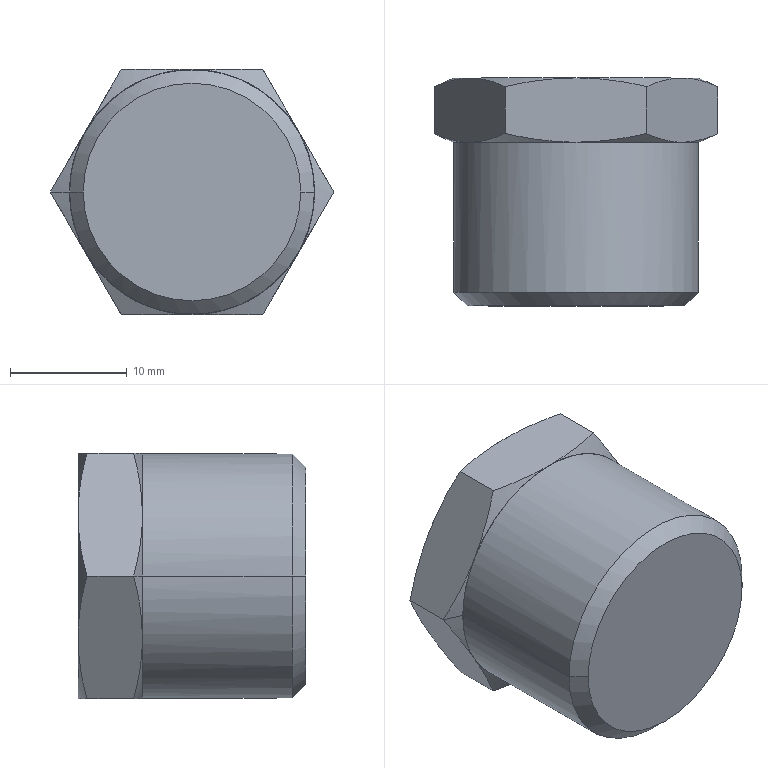Part | SolidWorks | features BaseBody 1 | 1 solid | 27 faces | box 24.249 x 19.5 x 21 mm | volume 6870 mm3 | cone 16 | plane 9 | cylinder 2 | commonest cylinder face diameters 20.955 x2
STEP:
#1=CARTESIAN_POINT('',(9.093,19.5,-5.25));
#2=VERTEX_POINT('',#1);
#3=CARTESIAN_POINT('',(10.5,19.5,0.));
#4=VERTEX_POINT('',#3);
#5=CARTESIAN_POINT('',(0.,19.5,0.));
#6=DIRECTION('',(0.,-1.,0.));
#7=DIRECTION('',(1.,0.,0.));
#8=AXIS2_PLACEMENT_3D('',#5,#6,#7);
#9=CIRCLE('',#8,10.5);
#10=EDGE_CURVE('',#2,#4,#9,.T.);
#11=ORIENTED_EDGE('',*,*,#10,.T.);
#12=CARTESIAN_POINT('',(12.124,18.76,0.));
#13=VERTEX_POINT('',#12);
#14=CARTESIAN_POINT('',(10.5,19.5,0.));
#15=DIRECTION('',(0.91,-0.4147,0.));
#16=VECTOR('',#15,1000.);
#17=LINE('',#14,#16);
#18=EDGE_CURVE('',#4,#13,#17,.T.);
#19=ORIENTED_EDGE('',*,*,#18,.T.);
#20=CARTESIAN_POINT('',(12.124,18.76,0.));
#21=CARTESIAN_POINT('',(11.626,18.987,-0.864));
#22=CARTESIAN_POINT('',(11.124,19.174,-1.732));
#23=CARTESIAN_POINT('',(10.114,19.43,-3.481));
#24=CARTESIAN_POINT('',(9.606,19.5,-4.362));
#25=CARTESIAN_POINT('',(9.093,19.5,-5.25));
#26=B_SPLINE_CURVE_WITH_KNOTS('',3,(#20,#21,#22,#23,#24,#25),.UNSPECIFIED.,.F.,.F.,(4,2,4),(0.,0.003054,0.006107),.UNSPECIFIED.);
#27=EDGE_CURVE('',#13,#2,#26,.T.);
#28=ORIENTED_EDGE('',*,*,#27,.T.);
#29=EDGE_LOOP('',(#11,#19,#28));
#30=FACE_OUTER_BOUND('',#29,.T.);
#31=CARTESIAN_POINT('',(0.,19.5,0.));
#32=DIRECTION('',(0.,-1.,0.));
#33=DIRECTION('',(1.,0.,0.));
#34=AXIS2_PLACEMENT_3D('',#31,#32,#33);
#35=CONICAL_SURFACE('',#34,10.5,1.143);
#36=ADVANCED_FACE('',(#30),#35,.T.);
#37=CARTESIAN_POINT('',(-10.5,14.,0.));
#38=VERTEX_POINT('',#37);
#39=CARTESIAN_POINT('',(-9.093,14.,-5.25));
#40=VERTEX_POINT('',#39);
#41=CARTESIAN_POINT('',(0.,14.,0.));
#42=DIRECTION('',(0.,-1.,0.));
#43=DIRECTION('',(1.,0.,0.));
#44=AXIS2_PLACEMENT_3D('',#41,#42,#43);
#45=CIRCLE('',#44,10.5);
#46=EDGE_CURVE('',#38,#40,#45,.T.);
#47=ORIENTED_EDGE('',*,*,#46,.F.);
#48=CARTESIAN_POINT('',(-12.124,14.74,0.));
#49=VERTEX_POINT('',#48);
#50=CARTESIAN_POINT('',(-12.124,14.74,0.));
#51=DIRECTION('',(-0.91,0.4147,0.));
#52=VECTOR('',#51,1000.);
#53=LINE('',#50,#52);
#54=EDGE_CURVE('',#38,#49,#53,.T.);
#55=ORIENTED_EDGE('',*,*,#54,.T.);
#56=CARTESIAN_POINT('',(-12.124,14.74,0.));
#57=CARTESIAN_POINT('',(-11.626,14.513,-0.864));
#58=CARTESIAN_POINT('',(-11.124,14.326,-1.732));
#59=CARTESIAN_POINT('',(-10.114,14.07,-3.481));
#60=CARTESIAN_POINT('',(-9.606,14.,-4.362));
#61=CARTESIAN_POINT('',(-9.093,14.,-5.25));
#62=B_SPLINE_CURVE_WITH_KNOTS('',3,(#56,#57,#58,#59,#60,#61),.UNSPECIFIED.,.F.,.F.,(4,2,4),(0.,0.003054,0.006107),.UNSPECIFIED.);
#63=EDGE_CURVE('',#49,#40,#62,.T.);
#64=ORIENTED_EDGE('',*,*,#63,.T.);
#65=EDGE_LOOP('',(#47,#55,#64));
#66=FACE_OUTER_BOUND('',#65,.T.);
#67=CARTESIAN_POINT('',(0.,14.74,0.));
#68=DIRECTION('',(0.,1.,0.));
#69=DIRECTION('',(-1.,0.,0.));
#70=AXIS2_PLACEMENT_3D('',#67,#68,#69);
#71=CONICAL_SURFACE('',#70,12.124,1.143);
#72=ADVANCED_FACE('',(#66),#71,.T.);
#73=CARTESIAN_POINT('',(-10.478,1.162,0.));
#74=VERTEX_POINT('',#73);
#75=CARTESIAN_POINT('',(10.478,1.162,0.));
#76=VERTEX_POINT('',#75);
#77=CARTESIAN_POINT('',(0.,1.162,0.));
#78=DIRECTION('',(0.,-1.,0.));
#79=DIRECTION('',(1.,0.,0.));
#80=AXIS2_PLACEMENT_3D('',#77,#78,#79);
#81=CIRCLE('',#80,10.478);
#82=EDGE_CURVE('',#74,#76,#81,.T.);
#83=ORIENTED_EDGE('',*,*,#82,.F.);
#84=CARTESIAN_POINT('',(-10.478,14.,0.));
#85=VERTEX_POINT('',#84);
#86=CARTESIAN_POINT('',(-10.478,0.,0.));
#87=DIRECTION('',(0.,1.,0.));
#88=VECTOR('',#87,1000.);
#89=LINE('',#86,#88);
#90=EDGE_CURVE('',#74,#85,#89,.T.);
#91=ORIENTED_EDGE('',*,*,#90,.T.);
#92=CARTESIAN_POINT('',(10.477,14.,0.));
#93=VERTEX_POINT('',#92);
#94=CARTESIAN_POINT('',(0.,14.,0.));
#95=DIRECTION('',(0.,-1.,0.));
#96=DIRECTION('',(1.,0.,0.));
#97=AXIS2_PLACEMENT_3D('',#94,#95,#96);
#98=CIRCLE('',#97,10.478);
#99=EDGE_CURVE('',#85,#93,#98,.T.);
#100=ORIENTED_EDGE('',*,*,#99,.T.);
#101=CARTESIAN_POINT('',(10.478,0.,0.));
#102=DIRECTION('',(0.,1.,0.));
#103=VECTOR('',#102,1000.);
#104=LINE('',#101,#103);
#105=EDGE_CURVE('',#76,#93,#104,.T.);
#106=ORIENTED_EDGE('',*,*,#105,.F.);
#107=EDGE_LOOP('',(#83,#91,#100,#106));
#108=FACE_OUTER_BOUND('',#107,.T.);
#109=CARTESIAN_POINT('',(0.,0.,0.));
#110=DIRECTION('',(0.,1.,0.));
#111=DIRECTION('',(1.,0.,0.));
#112=AXIS2_PLACEMENT_3D('',#109,#110,#111);
#113=CYLINDRICAL_SURFACE('',#112,10.478);
#114=ADVANCED_FACE('',(#108),#113,.T.);
#115=CARTESIAN_POINT('',(9.316,0.,0.));
#116=VERTEX_POINT('',#115);
#117=CARTESIAN_POINT('',(-9.316,0.,0.));
#118=VERTEX_POINT('',#117);
#119=CARTESIAN_POINT('',(0.,0.,0.));
#120=DIRECTION('',(0.,-1.,0.));
#121=DIRECTION('',(1.,0.,0.));
#122=AXIS2_PLACEMENT_3D('',#119,#120,#121);
#123=CIRCLE('',#122,9.316);
#124=EDGE_CURVE('',#116,#118,#123,.T.);
#125=ORIENTED_EDGE('',*,*,#124,.F.);
#126=CARTESIAN_POINT('',(10.478,1.162,0.));
#127=DIRECTION('',(0.7071,0.7071,0.));
#128=VECTOR('',#127,1000.);
#129=LINE('',#126,#128);
#130=EDGE_CURVE('',#116,#76,#129,.T.);
#131=ORIENTED_EDGE('',*,*,#130,.T.);
#132=CARTESIAN_POINT('',(0.,1.162,0.));
#133=DIRECTION('',(0.,-1.,0.));
#134=DIRECTION('',(1.,0.,0.));
#135=AXIS2_PLACEMENT_3D('',#132,#133,#134);
#136=CIRCLE('',#135,10.478);
#137=EDGE_CURVE('',#76,#74,#136,.T.);
#138=ORIENTED_EDGE('',*,*,#137,.T.);
#139=CARTESIAN_POINT('',(-10.478,1.162,0.));
#140=DIRECTION('',(-0.7071,0.7071,0.));
#141=VECTOR('',#140,1000.);
#142=LINE('',#139,#141);
#143=EDGE_CURVE('',#118,#74,#142,.T.);
#144=ORIENTED_EDGE('',*,*,#143,.F.);
#145=EDGE_LOOP('',(#125,#131,#138,#144));
#146=FACE_OUTER_BOUND('',#145,.T.);
#147=CARTESIAN_POINT('',(0.,1.162,0.));
#148=DIRECTION('',(0.,1.,0.));
#149=DIRECTION('',(-1.,0.,0.));
#150=AXIS2_PLACEMENT_3D('',#147,#148,#149);
#151=CONICAL_SURFACE('',#150,10.478,0.7854);
#152=ADVANCED_FACE('',(#146),#151,.T.);
#153=CARTESIAN_POINT('',(0.,14.,0.));
#154=DIRECTION('',(0.,-1.,0.));
#155=DIRECTION('',(1.,0.,0.));
#156=AXIS2_PLACEMENT_3D('',#153,#154,#155);
#157=CIRCLE('',#156,10.478);
#158=EDGE_CURVE('',#93,#85,#157,.T.);
#159=ORIENTED_EDGE('',*,*,#158,.F.);
#160=ORIENTED_EDGE('',*,*,#99,.F.);
#161=EDGE_LOOP('',(#159,#160));
#162=FACE_BOUND('',#161,.T.);
#163=CARTESIAN_POINT('',(0.,14.,-10.5));
#164=VERTEX_POINT('',#163);
#165=CARTESIAN_POINT('',(9.093,14.,-5.25));
#166=VERTEX_POINT('',#165);
#167=CARTESIAN_POINT('',(0.,14.,0.));
#168=DIRECTION('',(0.,-1.,0.));
#169=DIRECTION('',(1.,0.,0.));
#170=AXIS2_PLACEMENT_3D('',#167,#168,#169);
#171=CIRCLE('',#170,10.5);
#172=EDGE_CURVE('',#164,#166,#171,.T.);
#173=ORIENTED_EDGE('',*,*,#172,.T.);
#174=CARTESIAN_POINT('',(9.093,14.,5.25));
#175=VERTEX_POINT('',#174);
#176=CARTESIAN_POINT('',(0.,14.,0.));
#177=DIRECTION('',(0.,-1.,0.));
#178=DIRECTION('',(1.,0.,0.));
#179=AXIS2_PLACEMENT_3D('',#176,#177,#178);
#180=CIRCLE('',#179,10.5);
#181=EDGE_CURVE('',#166,#175,#180,.T.);
#182=ORIENTED_EDGE('',*,*,#181,.T.);
#183=CARTESIAN_POINT('',(0.,14.,10.5));
#184=VERTEX_POINT('',#183);
#185=CARTESIAN_POINT('',(0.,14.,0.));
#186=DIRECTION('',(0.,-1.,0.));
#187=DIRECTION('',(1.,0.,0.));
#188=AXIS2_PLACEMENT_3D('',#185,#186,#187);
#189=CIRCLE('',#188,10.5);
#190=EDGE_CURVE('',#175,#184,#189,.T.);
#191=ORIENTED_EDGE('',*,*,#190,.T.);
#192=CARTESIAN_POINT('',(-9.093,14.,5.25));
#193=VERTEX_POINT('',#192);
#194=CARTESIAN_POINT('',(0.,14.,0.));
#195=DIRECTION('',(0.,-1.,0.));
#196=DIRECTION('',(1.,0.,0.));
#197=AXIS2_PLACEMENT_3D('',#194,#195,#196);
#198=CIRCLE('',#197,10.5);
#199=EDGE_CURVE('',#184,#193,#198,.T.);
#200=ORIENTED_EDGE('',*,*,#199,.T.);
#201=CARTESIAN_POINT('',(0.,14.,0.));
#202=DIRECTION('',(0.,-1.,0.));
#203=DIRECTION('',(1.,0.,0.));
#204=AXIS2_PLACEMENT_3D('',#201,#202,#203);
#205=CIRCLE('',#204,10.5);
#206=EDGE_CURVE('',#193,#38,#205,.T.);
#207=ORIENTED_EDGE('',*,*,#206,.T.);
#208=ORIENTED_EDGE('',*,*,#46,.T.);
#209=CARTESIAN_POINT('',(0.,14.,0.));
#210=DIRECTION('',(0.,-1.,0.));
#211=DIRECTION('',(1.,0.,0.));
#212=AXIS2_PLACEMENT_3D('',#209,#210,#211);
#213=CIRCLE('',#212,10.5);
#214=EDGE_CURVE('',#40,#164,#213,.T.);
#215=ORIENTED_EDGE('',*,*,#214,.T.);
#216=EDGE_LOOP('',(#173,#182,#191,#200,#207,#208,#215));
#217=FACE_OUTER_BOUND('',#216,.T.);
#218=CARTESIAN_POINT('',(10.5,14.,0.));
#219=DIRECTION('',(0.,1.,0.));
#220=DIRECTION('',(0.,0.,-1.));
#221=AXIS2_PLACEMENT_3D('',#218,#219,#220);
#222=PLANE('',#221);
#223=ADVANCED_FACE('',(#162,#217),#222,.F.);
#224=ORIENTED_EDGE('',*,*,#199,.F.);
#225=CARTESIAN_POINT('',(-6.062,14.74,10.5));
#226=VERTEX_POINT('',#225);
#227=CARTESIAN_POINT('',(0.,14.,10.5));
#228=CARTESIAN_POINT('',(-1.025,14.,10.5));
#229=CARTESIAN_POINT('',(-2.042,14.07,10.5));
#230=CARTESIAN_POINT('',(-4.062,14.326,10.5));
#231=CARTESIAN_POINT('',(-5.065,14.513,10.5));
#232=CARTESIAN_POINT('',(-6.062,14.74,10.5));
#233=B_SPLINE_CURVE_WITH_KNOTS('',3,(#227,#228,#229,#230,#231,#232),.UNSPECIFIED.,.F.,.F.,(4,2,4),(0.,0.003054,0.006107),.UNSPECIFIED.);
#234=EDGE_CURVE('',#184,#226,#233,.T.);
#235=ORIENTED_EDGE('',*,*,#234,.T.);
#236=CARTESIAN_POINT('',(-6.062,14.74,10.5));
#237=CARTESIAN_POINT('',(-6.561,14.513,9.636));
#238=CARTESIAN_POINT('',(-7.062,14.326,8.768));
#239=CARTESIAN_POINT('',(-8.072,14.07,7.019));
#240=CARTESIAN_POINT('',(-8.581,14.,6.138));
#241=CARTESIAN_POINT('',(-9.093,14.,5.25));
#242=B_SPLINE_CURVE_WITH_KNOTS('',3,(#236,#237,#238,#239,#240,#241),.UNSPECIFIED.,.F.,.F.,(4,2,4),(0.,0.003054,0.006107),.UNSPECIFIED.);
#243=EDGE_CURVE('',#226,#193,#242,.T.);
#244=ORIENTED_EDGE('',*,*,#243,.T.);
#245=EDGE_LOOP('',(#224,#235,#244));
#246=FACE_OUTER_BOUND('',#245,.T.);
#247=CARTESIAN_POINT('',(0.,14.74,0.));
#248=DIRECTION('',(0.,1.,0.));
#249=DIRECTION('',(-1.,0.,0.));
#250=AXIS2_PLACEMENT_3D('',#247,#248,#249);
#251=CONICAL_SURFACE('',#250,12.124,1.143);
#252=ADVANCED_FACE('',(#246),#251,.T.);
#253=CARTESIAN_POINT('',(12.124,14.74,0.));
#254=VERTEX_POINT('',#253);
#255=CARTESIAN_POINT('',(12.124,19.5,0.));
#256=DIRECTION('',(0.,-1.,0.));
#257=VECTOR('',#256,1000.);
#258=LINE('',#255,#257);
#259=EDGE_CURVE('',#13,#254,#258,.T.);
#260=ORIENTED_EDGE('',*,*,#259,.T.);
#261=CARTESIAN_POINT('',(9.093,14.,-5.25));
#262=CARTESIAN_POINT('',(9.606,14.,-4.362));
#263=CARTESIAN_POINT('',(10.114,14.07,-3.481));
#264=CARTESIAN_POINT('',(11.124,14.326,-1.732));
#265=CARTESIAN_POINT('',(11.626,14.513,-0.864));
#266=CARTESIAN_POINT('',(12.124,14.74,0.));
#267=B_SPLINE_CURVE_WITH_KNOTS('',3,(#261,#262,#263,#264,#265,#266),.UNSPECIFIED.,.F.,.F.,(4,2,4),(0.,0.003054,0.006107),.UNSPECIFIED.);
#268=EDGE_CURVE('',#166,#254,#267,.T.);
#269=ORIENTED_EDGE('',*,*,#268,.F.);
#270=CARTESIAN_POINT('',(6.062,14.74,-10.5));
#271=VERTEX_POINT('',#270);
#272=CARTESIAN_POINT('',(6.062,14.74,-10.5));
#273=CARTESIAN_POINT('',(6.561,14.513,-9.636));
#274=CARTESIAN_POINT('',(7.062,14.326,-8.768));
#275=CARTESIAN_POINT('',(8.072,14.07,-7.019));
#276=CARTESIAN_POINT('',(8.581,14.,-6.138));
#277=CARTESIAN_POINT('',(9.093,14.,-5.25));
#278=B_SPLINE_CURVE_WITH_KNOTS('',3,(#272,#273,#274,#275,#276,#277),.UNSPECIFIED.,.F.,.F.,(4,2,4),(0.,0.003054,0.006107),.UNSPECIFIED.);
#279=EDGE_CURVE('',#271,#166,#278,.T.);
#280=ORIENTED_EDGE('',*,*,#279,.F.);
#281=CARTESIAN_POINT('',(6.062,18.76,-10.5));
#282=VERTEX_POINT('',#281);
#283=CARTESIAN_POINT('',(6.062,19.5,-10.5));
#284=DIRECTION('',(0.,-1.,0.));
#285=VECTOR('',#284,1000.);
#286=LINE('',#283,#285);
#287=EDGE_CURVE('',#282,#271,#286,.T.);
#288=ORIENTED_EDGE('',*,*,#287,.F.);
#289=CARTESIAN_POINT('',(9.093,19.5,-5.25));
#290=CARTESIAN_POINT('',(8.581,19.5,-6.138));
#291=CARTESIAN_POINT('',(8.072,19.43,-7.019));
#292=CARTESIAN_POINT('',(7.062,19.174,-8.768));
#293=CARTESIAN_POINT('',(6.561,18.987,-9.636));
#294=CARTESIAN_POINT('',(6.062,18.76,-10.5));
#295=B_SPLINE_CURVE_WITH_KNOTS('',3,(#289,#290,#291,#292,#293,#294),.UNSPECIFIED.,.F.,.F.,(4,2,4),(0.,0.003054,0.006107),.UNSPECIFIED.);
#296=EDGE_CURVE('',#2,#282,#295,.T.);
#297=ORIENTED_EDGE('',*,*,#296,.F.);
#298=ORIENTED_EDGE('',*,*,#27,.F.);
#299=EDGE_LOOP('',(#260,#269,#280,#288,#297,#298));
#300=FACE_OUTER_BOUND('',#299,.T.);
#301=CARTESIAN_POINT('',(12.124,19.5,0.));
#302=DIRECTION('',(-0.866,0.,0.5));
#303=DIRECTION('',(0.,1.,0.));
#304=AXIS2_PLACEMENT_3D('',#301,#302,#303);
#305=PLANE('',#304);
#306=ADVANCED_FACE('',(#300),#305,.F.);
#307=CARTESIAN_POINT('',(-9.093,19.5,5.25));
#308=VERTEX_POINT('',#307);
#309=CARTESIAN_POINT('',(-6.062,18.76,10.5));
#310=VERTEX_POINT('',#309);
#311=CARTESIAN_POINT('',(-9.093,19.5,5.25));
#312=CARTESIAN_POINT('',(-8.581,19.5,6.138));
#313=CARTESIAN_POINT('',(-8.072,19.43,7.019));
#314=CARTESIAN_POINT('',(-7.062,19.174,8.768));
#315=CARTESIAN_POINT('',(-6.561,18.987,9.636));
#316=CARTESIAN_POINT('',(-6.062,18.76,10.5));
#317=B_SPLINE_CURVE_WITH_KNOTS('',3,(#311,#312,#313,#314,#315,#316),.UNSPECIFIED.,.F.,.F.,(4,2,4),(0.,0.003054,0.006107),.UNSPECIFIED.);
#318=EDGE_CURVE('',#308,#310,#317,.T.);
#319=ORIENTED_EDGE('',*,*,#318,.T.);
#320=CARTESIAN_POINT('',(0.,19.5,10.5));
#321=VERTEX_POINT('',#320);
#322=CARTESIAN_POINT('',(-6.062,18.76,10.5));
#323=CARTESIAN_POINT('',(-5.065,18.987,10.5));
#324=CARTESIAN_POINT('',(-4.062,19.174,10.5));
#325=CARTESIAN_POINT('',(-2.042,19.43,10.5));
#326=CARTESIAN_POINT('',(-1.025,19.5,10.5));
#327=CARTESIAN_POINT('',(0.,19.5,10.5));
#328=B_SPLINE_CURVE_WITH_KNOTS('',3,(#322,#323,#324,#325,#326,#327),.UNSPECIFIED.,.F.,.F.,(4,2,4),(0.,0.003054,0.006107),.UNSPECIFIED.);
#329=EDGE_CURVE('',#310,#321,#328,.T.);
#330=ORIENTED_EDGE('',*,*,#329,.T.);
#331=CARTESIAN_POINT('',(0.,19.5,0.));
#332=DIRECTION('',(0.,-1.,0.));
#333=DIRECTION('',(1.,0.,0.));
#334=AXIS2_PLACEMENT_3D('',#331,#332,#333);
#335=CIRCLE('',#334,10.5);
#336=EDGE_CURVE('',#321,#308,#335,.T.);
#337=ORIENTED_EDGE('',*,*,#336,.T.);
#338=EDGE_LOOP('',(#319,#330,#337));
#339=FACE_OUTER_BOUND('',#338,.T.);
#340=CARTESIAN_POINT('',(0.,19.5,0.));
#341=DIRECTION('',(0.,-1.,0.));
#342=DIRECTION('',(1.,0.,0.));
#343=AXIS2_PLACEMENT_3D('',#340,#341,#342);
#344=CONICAL_SURFACE('',#343,10.5,1.143);
#345=ADVANCED_FACE('',(#339),#344,.T.);
#346=ORIENTED_EDGE('',*,*,#10,.F.);
#347=CARTESIAN_POINT('',(0.,19.5,-10.5));
#348=VERTEX_POINT('',#347);
#349=CARTESIAN_POINT('',(0.,19.5,0.));
#350=DIRECTION('',(0.,-1.,0.));
#351=DIRECTION('',(1.,0.,0.));
#352=AXIS2_PLACEMENT_3D('',#349,#350,#351);
#353=CIRCLE('',#352,10.5);
#354=EDGE_CURVE('',#348,#2,#353,.T.);
#355=ORIENTED_EDGE('',*,*,#354,.F.);
#356=CARTESIAN_POINT('',(-9.093,19.5,-5.25));
#357=VERTEX_POINT('',#356);
#358=CARTESIAN_POINT('',(0.,19.5,0.));
#359=DIRECTION('',(0.,-1.,0.));
#360=DIRECTION('',(1.,0.,0.));
#361=AXIS2_PLACEMENT_3D('',#358,#359,#360);
#362=CIRCLE('',#361,10.5);
#363=EDGE_CURVE('',#357,#348,#362,.T.);
#364=ORIENTED_EDGE('',*,*,#363,.F.);
#365=CARTESIAN_POINT('',(0.,19.5,0.));
#366=DIRECTION('',(0.,-1.,0.));
#367=DIRECTION('',(1.,0.,0.));
#368=AXIS2_PLACEMENT_3D('',#365,#366,#367);
#369=CIRCLE('',#368,10.5);
#370=EDGE_CURVE('',#308,#357,#369,.T.);
#371=ORIENTED_EDGE('',*,*,#370,.F.);
#372=ORIENTED_EDGE('',*,*,#336,.F.);
#373=CARTESIAN_POINT('',(9.093,19.5,5.25));
#374=VERTEX_POINT('',#373);
#375=CARTESIAN_POINT('',(0.,19.5,0.));
#376=DIRECTION('',(0.,-1.,0.));
#377=DIRECTION('',(1.,0.,0.));
#378=AXIS2_PLACEMENT_3D('',#375,#376,#377);
#379=CIRCLE('',#378,10.5);
#380=EDGE_CURVE('',#374,#321,#379,.T.);
#381=ORIENTED_EDGE('',*,*,#380,.F.);
#382=CARTESIAN_POINT('',(0.,19.5,0.));
#383=DIRECTION('',(0.,-1.,0.));
#384=DIRECTION('',(1.,0.,0.));
#385=AXIS2_PLACEMENT_3D('',#382,#383,#384);
#386=CIRCLE('',#385,10.5);
#387=EDGE_CURVE('',#4,#374,#386,.T.);
#388=ORIENTED_EDGE('',*,*,#387,.F.);
#389=EDGE_LOOP('',(#346,#355,#364,#371,#372,#381,#388));
#390=FACE_OUTER_BOUND('',#389,.T.);
#391=CARTESIAN_POINT('',(0.,19.5,0.));
#392=DIRECTION('',(0.,-1.,0.));
#393=DIRECTION('',(0.,0.,-1.));
#394=AXIS2_PLACEMENT_3D('',#391,#392,#393);
#395=PLANE('',#394);
#396=ADVANCED_FACE('',(#390),#395,.F.);
#397=CARTESIAN_POINT('',(6.062,18.76,10.5));
#398=VERTEX_POINT('',#397);
#399=CARTESIAN_POINT('',(0.,19.5,10.5));
#400=CARTESIAN_POINT('',(1.025,19.5,10.5));
#401=CARTESIAN_POINT('',(2.042,19.43,10.5));
#402=CARTESIAN_POINT('',(4.062,19.174,10.5));
#403=CARTESIAN_POINT('',(5.065,18.987,10.5));
#404=CARTESIAN_POINT('',(6.062,18.76,10.5));
#405=B_SPLINE_CURVE_WITH_KNOTS('',3,(#399,#400,#401,#402,#403,#404),.UNSPECIFIED.,.F.,.F.,(4,2,4),(0.,0.003054,0.006107),.UNSPECIFIED.);
#406=EDGE_CURVE('',#321,#398,#405,.T.);
#407=ORIENTED_EDGE('',*,*,#406,.T.);
#408=CARTESIAN_POINT('',(6.062,18.76,10.5));
#409=CARTESIAN_POINT('',(6.561,18.987,9.636));
#410=CARTESIAN_POINT('',(7.062,19.174,8.768));
#411=CARTESIAN_POINT('',(8.072,19.43,7.019));
#412=CARTESIAN_POINT('',(8.581,19.5,6.138));
#413=CARTESIAN_POINT('',(9.093,19.5,5.25));
#414=B_SPLINE_CURVE_WITH_KNOTS('',3,(#408,#409,#410,#411,#412,#413),.UNSPECIFIED.,.F.,.F.,(4,2,4),(0.,0.003054,0.006107),.UNSPECIFIED.);
#415=EDGE_CURVE('',#398,#374,#414,.T.);
#416=ORIENTED_EDGE('',*,*,#415,.T.);
#417=ORIENTED_EDGE('',*,*,#380,.T.);
#418=EDGE_LOOP('',(#407,#416,#417));
#419=FACE_OUTER_BOUND('',#418,.T.);
#420=CARTESIAN_POINT('',(0.,19.5,0.));
#421=DIRECTION('',(0.,-1.,0.));
#422=DIRECTION('',(1.,0.,0.));
#423=AXIS2_PLACEMENT_3D('',#420,#421,#422);
#424=CONICAL_SURFACE('',#423,10.5,1.143);
#425=ADVANCED_FACE('',(#419),#424,.T.);
#426=ORIENTED_EDGE('',*,*,#370,.T.);
#427=CARTESIAN_POINT('',(-12.124,18.76,0.));
#428=VERTEX_POINT('',#427);
#429=CARTESIAN_POINT('',(-9.093,19.5,-5.25));
#430=CARTESIAN_POINT('',(-9.606,19.5,-4.362));
#431=CARTESIAN_POINT('',(-10.114,19.43,-3.481));
#432=CARTESIAN_POINT('',(-11.124,19.174,-1.732));
#433=CARTESIAN_POINT('',(-11.626,18.987,-0.864));
#434=CARTESIAN_POINT('',(-12.124,18.76,0.));
#435=B_SPLINE_CURVE_WITH_KNOTS('',3,(#429,#430,#431,#432,#433,#434),.UNSPECIFIED.,.F.,.F.,(4,2,4),(0.,0.003054,0.006107),.UNSPECIFIED.);
#436=EDGE_CURVE('',#357,#428,#435,.T.);
#437=ORIENTED_EDGE('',*,*,#436,.T.);
#438=CARTESIAN_POINT('',(-12.124,18.76,0.));
#439=CARTESIAN_POINT('',(-11.626,18.987,0.864));
#440=CARTESIAN_POINT('',(-11.124,19.174,1.732));
#441=CARTESIAN_POINT('',(-10.114,19.43,3.481));
#442=CARTESIAN_POINT('',(-9.606,19.5,4.362));
#443=CARTESIAN_POINT('',(-9.093,19.5,5.25));
#444=B_SPLINE_CURVE_WITH_KNOTS('',3,(#438,#439,#440,#441,#442,#443),.UNSPECIFIED.,.F.,.F.,(4,2,4),(0.,0.003054,0.006107),.UNSPECIFIED.);
#445=EDGE_CURVE('',#428,#308,#444,.T.);
#446=ORIENTED_EDGE('',*,*,#445,.T.);
#447=EDGE_LOOP('',(#426,#437,#446));
#448=FACE_OUTER_BOUND('',#447,.T.);
#449=CARTESIAN_POINT('',(0.,19.5,0.));
#450=DIRECTION('',(0.,-1.,0.));
#451=DIRECTION('',(1.,0.,0.));
#452=AXIS2_PLACEMENT_3D('',#449,#450,#451);
#453=CONICAL_SURFACE('',#452,10.5,1.143);
#454=ADVANCED_FACE('',(#448),#453,.T.);
#455=ORIENTED_EDGE('',*,*,#354,.T.);
#456=ORIENTED_EDGE('',*,*,#296,.T.);
#457=CARTESIAN_POINT('',(6.062,18.76,-10.5));
#458=CARTESIAN_POINT('',(5.065,18.987,-10.5));
#459=CARTESIAN_POINT('',(4.062,19.174,-10.5));
#460=CARTESIAN_POINT('',(2.042,19.43,-10.5));
#461=CARTESIAN_POINT('',(1.025,19.5,-10.5));
#462=CARTESIAN_POINT('',(0.,19.5,-10.5));
#463=B_SPLINE_CURVE_WITH_KNOTS('',3,(#457,#458,#459,#460,#461,#462),.UNSPECIFIED.,.F.,.F.,(4,2,4),(0.,0.003054,0.006107),.UNSPECIFIED.);
#464=EDGE_CURVE('',#282,#348,#463,.T.);
#465=ORIENTED_EDGE('',*,*,#464,.T.);
#466=EDGE_LOOP('',(#455,#456,#465));
#467=FACE_OUTER_BOUND('',#466,.T.);
#468=CARTESIAN_POINT('',(0.,19.5,0.));
#469=DIRECTION('',(0.,-1.,0.));
#470=DIRECTION('',(1.,0.,0.));
#471=AXIS2_PLACEMENT_3D('',#468,#469,#470);
#472=CONICAL_SURFACE('',#471,10.5,1.143);
#473=ADVANCED_FACE('',(#467),#472,.T.);
#474=ORIENTED_EDGE('',*,*,#363,.T.);
#475=CARTESIAN_POINT('',(-6.062,18.76,-10.5));
#476=VERTEX_POINT('',#475);
#477=CARTESIAN_POINT('',(0.,19.5,-10.5));
#478=CARTESIAN_POINT('',(-1.025,19.5,-10.5));
#479=CARTESIAN_POINT('',(-2.042,19.43,-10.5));
#480=CARTESIAN_POINT('',(-4.062,19.174,-10.5));
#481=CARTESIAN_POINT('',(-5.065,18.987,-10.5));
#482=CARTESIAN_POINT('',(-6.062,18.76,-10.5));
#483=B_SPLINE_CURVE_WITH_KNOTS('',3,(#477,#478,#479,#480,#481,#482),.UNSPECIFIED.,.F.,.F.,(4,2,4),(0.,0.003054,0.006107),.UNSPECIFIED.);
#484=EDGE_CURVE('',#348,#476,#483,.T.);
#485=ORIENTED_EDGE('',*,*,#484,.T.);
#486=CARTESIAN_POINT('',(-6.062,18.76,-10.5));
#487=CARTESIAN_POINT('',(-6.561,18.987,-9.636));
#488=CARTESIAN_POINT('',(-7.062,19.174,-8.768));
#489=CARTESIAN_POINT('',(-8.072,19.43,-7.019));
#490=CARTESIAN_POINT('',(-8.581,19.5,-6.138));
#491=CARTESIAN_POINT('',(-9.093,19.5,-5.25));
#492=B_SPLINE_CURVE_WITH_KNOTS('',3,(#486,#487,#488,#489,#490,#491),.UNSPECIFIED.,.F.,.F.,(4,2,4),(0.,0.003054,0.006107),.UNSPECIFIED.);
#493=EDGE_CURVE('',#476,#357,#492,.T.);
#494=ORIENTED_EDGE('',*,*,#493,.T.);
#495=EDGE_LOOP('',(#474,#485,#494));
#496=FACE_OUTER_BOUND('',#495,.T.);
#497=CARTESIAN_POINT('',(0.,19.5,0.));
#498=DIRECTION('',(0.,-1.,0.));
#499=DIRECTION('',(1.,0.,0.));
#500=AXIS2_PLACEMENT_3D('',#497,#498,#499);
#501=CONICAL_SURFACE('',#500,10.5,1.143);
#502=ADVANCED_FACE('',(#496),#501,.T.);
#503=ORIENTED_EDGE('',*,*,#190,.F.);
#504=CARTESIAN_POINT('',(6.062,14.74,10.5));
#505=VERTEX_POINT('',#504);
#506=CARTESIAN_POINT('',(9.093,14.,5.25));
#507=CARTESIAN_POINT('',(8.581,14.,6.138));
#508=CARTESIAN_POINT('',(8.072,14.07,7.019));
#509=CARTESIAN_POINT('',(7.062,14.326,8.768));
#510=CARTESIAN_POINT('',(6.561,14.513,9.636));
#511=CARTESIAN_POINT('',(6.062,14.74,10.5));
#512=B_SPLINE_CURVE_WITH_KNOTS('',3,(#506,#507,#508,#509,#510,#511),.UNSPECIFIED.,.F.,.F.,(4,2,4),(0.,0.003054,0.006107),.UNSPECIFIED.);
#513=EDGE_CURVE('',#175,#505,#512,.T.);
#514=ORIENTED_EDGE('',*,*,#513,.T.);
#515=CARTESIAN_POINT('',(6.062,14.74,10.5));
#516=CARTESIAN_POINT('',(5.065,14.513,10.5));
#517=CARTESIAN_POINT('',(4.062,14.326,10.5));
#518=CARTESIAN_POINT('',(2.042,14.07,10.5));
#519=CARTESIAN_POINT('',(1.025,14.,10.5));
#520=CARTESIAN_POINT('',(0.,14.,10.5));
#521=B_SPLINE_CURVE_WITH_KNOTS('',3,(#515,#516,#517,#518,#519,#520),.UNSPECIFIED.,.F.,.F.,(4,2,4),(0.,0.003054,0.006107),.UNSPECIFIED.);
#522=EDGE_CURVE('',#505,#184,#521,.T.);
#523=ORIENTED_EDGE('',*,*,#522,.T.);
#524=EDGE_LOOP('',(#503,#514,#523));
#525=FACE_OUTER_BOUND('',#524,.T.);
#526=CARTESIAN_POINT('',(0.,14.74,0.));
#527=DIRECTION('',(0.,1.,0.));
#528=DIRECTION('',(-1.,0.,0.));
#529=AXIS2_PLACEMENT_3D('',#526,#527,#528);
#530=CONICAL_SURFACE('',#529,12.124,1.143);
#531=ADVANCED_FACE('',(#525),#530,.T.);
#532=ORIENTED_EDGE('',*,*,#172,.F.);
#533=CARTESIAN_POINT('',(0.,14.,-10.5));
#534=CARTESIAN_POINT('',(1.025,14.,-10.5));
#535=CARTESIAN_POINT('',(2.042,14.07,-10.5));
#536=CARTESIAN_POINT('',(4.062,14.326,-10.5));
#537=CARTESIAN_POINT('',(5.065,14.513,-10.5));
#538=CARTESIAN_POINT('',(6.062,14.74,-10.5));
#539=B_SPLINE_CURVE_WITH_KNOTS('',3,(#533,#534,#535,#536,#537,#538),.UNSPECIFIED.,.F.,.F.,(4,2,4),(0.,0.003054,0.006107),.UNSPECIFIED.);
#540=EDGE_CURVE('',#164,#271,#539,.T.);
#541=ORIENTED_EDGE('',*,*,#540,.T.);
#542=ORIENTED_EDGE('',*,*,#279,.T.);
#543=EDGE_LOOP('',(#532,#541,#542));
#544=FACE_OUTER_BOUND('',#543,.T.);
#545=CARTESIAN_POINT('',(0.,14.74,0.));
#546=DIRECTION('',(0.,1.,0.));
#547=DIRECTION('',(-1.,0.,0.));
#548=AXIS2_PLACEMENT_3D('',#545,#546,#547);
#549=CONICAL_SURFACE('',#548,12.124,1.143);
#550=ADVANCED_FACE('',(#544),#549,.T.);
#551=ORIENTED_EDGE('',*,*,#214,.F.);
#552=CARTESIAN_POINT('',(-6.062,14.74,-10.5));
#553=VERTEX_POINT('',#552);
#554=CARTESIAN_POINT('',(-9.093,14.,-5.25));
#555=CARTESIAN_POINT('',(-8.581,14.,-6.138));
#556=CARTESIAN_POINT('',(-8.072,14.07,-7.019));
#557=CARTESIAN_POINT('',(-7.062,14.326,-8.768));
#558=CARTESIAN_POINT('',(-6.561,14.513,-9.636));
#559=CARTESIAN_POINT('',(-6.062,14.74,-10.5));
#560=B_SPLINE_CURVE_WITH_KNOTS('',3,(#554,#555,#556,#557,#558,#559),.UNSPECIFIED.,.F.,.F.,(4,2,4),(0.,0.003054,0.006107),.UNSPECIFIED.);
#561=EDGE_CURVE('',#40,#553,#560,.T.);
#562=ORIENTED_EDGE('',*,*,#561,.T.);
#563=CARTESIAN_POINT('',(-6.062,14.74,-10.5));
#564=CARTESIAN_POINT('',(-5.065,14.513,-10.5));
#565=CARTESIAN_POINT('',(-4.062,14.326,-10.5));
#566=CARTESIAN_POINT('',(-2.042,14.07,-10.5));
#567=CARTESIAN_POINT('',(-1.025,14.,-10.5));
#568=CARTESIAN_POINT('',(0.,14.,-10.5));
#569=B_SPLINE_CURVE_WITH_KNOTS('',3,(#563,#564,#565,#566,#567,#568),.UNSPECIFIED.,.F.,.F.,(4,2,4),(0.,0.003054,0.006107),.UNSPECIFIED.);
#570=EDGE_CURVE('',#553,#164,#569,.T.);
#571=ORIENTED_EDGE('',*,*,#570,.T.);
#572=EDGE_LOOP('',(#551,#562,#571));
#573=FACE_OUTER_BOUND('',#572,.T.);
#574=CARTESIAN_POINT('',(0.,14.74,0.));
#575=DIRECTION('',(0.,1.,0.));
#576=DIRECTION('',(-1.,0.,0.));
#577=AXIS2_PLACEMENT_3D('',#574,#575,#576);
#578=CONICAL_SURFACE('',#577,12.124,1.143);
#579=ADVANCED_FACE('',(#573),#578,.T.);
#580=CARTESIAN_POINT('',(0.,0.,0.));
#581=DIRECTION('',(0.,-1.,0.));
#582=DIRECTION('',(1.,0.,0.));
#583=AXIS2_PLACEMENT_3D('',#580,#581,#582);
#584=CIRCLE('',#583,9.316);
#585=EDGE_CURVE('',#118,#116,#584,.T.);
#586=ORIENTED_EDGE('',*,*,#585,.T.);
#587=ORIENTED_EDGE('',*,*,#124,.T.);
#588=EDGE_LOOP('',(#586,#587));
#589=FACE_OUTER_BOUND('',#588,.T.);
#590=CARTESIAN_POINT('',(9.316,0.,0.));
#591=DIRECTION('',(0.,1.,0.));
#592=DIRECTION('',(0.,0.,-1.));
#593=AXIS2_PLACEMENT_3D('',#590,#591,#592);
#594=PLANE('',#593);
#595=ADVANCED_FACE('',(#589),#594,.F.);
#596=CARTESIAN_POINT('',(-12.124,19.5,0.));
#597=DIRECTION('',(0.,-1.,0.));
#598=VECTOR('',#597,1000.);
#599=LINE('',#596,#598);
#600=EDGE_CURVE('',#428,#49,#599,.T.);
#601=ORIENTED_EDGE('',*,*,#600,.T.);
#602=CARTESIAN_POINT('',(-9.093,14.,5.25));
#603=CARTESIAN_POINT('',(-9.606,14.,4.362));
#604=CARTESIAN_POINT('',(-10.114,14.07,3.481));
#605=CARTESIAN_POINT('',(-11.124,14.326,1.732));
#606=CARTESIAN_POINT('',(-11.626,14.513,0.864));
#607=CARTESIAN_POINT('',(-12.124,14.74,0.));
#608=B_SPLINE_CURVE_WITH_KNOTS('',3,(#602,#603,#604,#605,#606,#607),.UNSPECIFIED.,.F.,.F.,(4,2,4),(0.,0.003054,0.006107),.UNSPECIFIED.);
#609=EDGE_CURVE('',#193,#49,#608,.T.);
#610=ORIENTED_EDGE('',*,*,#609,.F.);
#611=ORIENTED_EDGE('',*,*,#243,.F.);
#612=CARTESIAN_POINT('',(-6.062,19.5,10.5));
#613=DIRECTION('',(0.,-1.,0.));
#614=VECTOR('',#613,1000.);
#615=LINE('',#612,#614);
#616=EDGE_CURVE('',#310,#226,#615,.T.);
#617=ORIENTED_EDGE('',*,*,#616,.F.);
#618=ORIENTED_EDGE('',*,*,#318,.F.);
#619=ORIENTED_EDGE('',*,*,#445,.F.);
#620=EDGE_LOOP('',(#601,#610,#611,#617,#618,#619));
#621=FACE_OUTER_BOUND('',#620,.T.);
#622=CARTESIAN_POINT('',(-12.124,19.5,0.));
#623=DIRECTION('',(0.866,0.,-0.5));
#624=DIRECTION('',(0.,-1.,0.));
#625=AXIS2_PLACEMENT_3D('',#622,#623,#624);
#626=PLANE('',#625);
#627=ADVANCED_FACE('',(#621),#626,.F.);
#628=ORIENTED_EDGE('',*,*,#616,.T.);
#629=ORIENTED_EDGE('',*,*,#234,.F.);
#630=ORIENTED_EDGE('',*,*,#522,.F.);
#631=CARTESIAN_POINT('',(6.062,19.5,10.5));
#632=DIRECTION('',(0.,-1.,0.));
#633=VECTOR('',#632,1000.);
#634=LINE('',#631,#633);
#635=EDGE_CURVE('',#398,#505,#634,.T.);
#636=ORIENTED_EDGE('',*,*,#635,.F.);
#637=ORIENTED_EDGE('',*,*,#406,.F.);
#638=ORIENTED_EDGE('',*,*,#329,.F.);
#639=EDGE_LOOP('',(#628,#629,#630,#636,#637,#638));
#640=FACE_OUTER_BOUND('',#639,.T.);
#641=CARTESIAN_POINT('',(-6.062,19.5,10.5));
#642=DIRECTION('',(0.,0.,-1.));
#643=DIRECTION('',(0.,-1.,0.));
#644=AXIS2_PLACEMENT_3D('',#641,#642,#643);
#645=PLANE('',#644);
#646=ADVANCED_FACE('',(#640),#645,.F.);
#647=ORIENTED_EDGE('',*,*,#635,.T.);
#648=ORIENTED_EDGE('',*,*,#513,.F.);
#649=CARTESIAN_POINT('',(12.124,14.74,0.));
#650=CARTESIAN_POINT('',(11.626,14.513,0.864));
#651=CARTESIAN_POINT('',(11.124,14.326,1.732));
#652=CARTESIAN_POINT('',(10.114,14.07,3.481));
#653=CARTESIAN_POINT('',(9.606,14.,4.362));
#654=CARTESIAN_POINT('',(9.093,14.,5.25));
#655=B_SPLINE_CURVE_WITH_KNOTS('',3,(#649,#650,#651,#652,#653,#654),.UNSPECIFIED.,.F.,.F.,(4,2,4),(0.,0.003054,0.006107),.UNSPECIFIED.);
#656=EDGE_CURVE('',#254,#175,#655,.T.);
#657=ORIENTED_EDGE('',*,*,#656,.F.);
#658=ORIENTED_EDGE('',*,*,#259,.F.);
#659=CARTESIAN_POINT('',(9.093,19.5,5.25));
#660=CARTESIAN_POINT('',(9.606,19.5,4.362));
#661=CARTESIAN_POINT('',(10.114,19.43,3.481));
#662=CARTESIAN_POINT('',(11.124,19.174,1.732));
#663=CARTESIAN_POINT('',(11.626,18.987,0.864));
#664=CARTESIAN_POINT('',(12.124,18.76,0.));
#665=B_SPLINE_CURVE_WITH_KNOTS('',3,(#659,#660,#661,#662,#663,#664),.UNSPECIFIED.,.F.,.F.,(4,2,4),(0.,0.003054,0.006107),.UNSPECIFIED.);
#666=EDGE_CURVE('',#374,#13,#665,.T.);
#667=ORIENTED_EDGE('',*,*,#666,.F.);
#668=ORIENTED_EDGE('',*,*,#415,.F.);
#669=EDGE_LOOP('',(#647,#648,#657,#658,#667,#668));
#670=FACE_OUTER_BOUND('',#669,.T.);
#671=CARTESIAN_POINT('',(6.062,19.5,10.5));
#672=DIRECTION('',(-0.866,0.,-0.5));
#673=DIRECTION('',(-0.5,0.,0.866));
#674=AXIS2_PLACEMENT_3D('',#671,#672,#673);
#675=PLANE('',#674);
#676=ADVANCED_FACE('',(#670),#675,.F.);
#677=ORIENTED_EDGE('',*,*,#181,.F.);
#678=ORIENTED_EDGE('',*,*,#268,.T.);
#679=ORIENTED_EDGE('',*,*,#656,.T.);
#680=EDGE_LOOP('',(#677,#678,#679));
#681=FACE_OUTER_BOUND('',#680,.T.);
#682=CARTESIAN_POINT('',(0.,14.74,0.));
#683=DIRECTION('',(0.,1.,0.));
#684=DIRECTION('',(-1.,0.,0.));
#685=AXIS2_PLACEMENT_3D('',#682,#683,#684);
#686=CONICAL_SURFACE('',#685,12.124,1.143);
#687=ADVANCED_FACE('',(#681),#686,.T.);
#688=ORIENTED_EDGE('',*,*,#287,.T.);
#689=ORIENTED_EDGE('',*,*,#540,.F.);
#690=ORIENTED_EDGE('',*,*,#570,.F.);
#691=CARTESIAN_POINT('',(-6.062,19.5,-10.5));
#692=DIRECTION('',(0.,-1.,0.));
#693=VECTOR('',#692,1000.);
#694=LINE('',#691,#693);
#695=EDGE_CURVE('',#476,#553,#694,.T.);
#696=ORIENTED_EDGE('',*,*,#695,.F.);
#697=ORIENTED_EDGE('',*,*,#484,.F.);
#698=ORIENTED_EDGE('',*,*,#464,.F.);
#699=EDGE_LOOP('',(#688,#689,#690,#696,#697,#698));
#700=FACE_OUTER_BOUND('',#699,.T.);
#701=CARTESIAN_POINT('',(6.062,19.5,-10.5));
#702=DIRECTION('',(0.,0.,1.));
#703=DIRECTION('',(1.,0.,0.));
#704=AXIS2_PLACEMENT_3D('',#701,#702,#703);
#705=PLANE('',#704);
#706=ADVANCED_FACE('',(#700),#705,.F.);
#707=ORIENTED_EDGE('',*,*,#695,.T.);
#708=ORIENTED_EDGE('',*,*,#561,.F.);
#709=ORIENTED_EDGE('',*,*,#63,.F.);
#710=ORIENTED_EDGE('',*,*,#600,.F.);
#711=ORIENTED_EDGE('',*,*,#436,.F.);
#712=ORIENTED_EDGE('',*,*,#493,.F.);
#713=EDGE_LOOP('',(#707,#708,#709,#710,#711,#712));
#714=FACE_OUTER_BOUND('',#713,.T.);
#715=CARTESIAN_POINT('',(-6.062,19.5,-10.5));
#716=DIRECTION('',(0.866,0.,0.5));
#717=DIRECTION('',(0.,-1.,0.));
#718=AXIS2_PLACEMENT_3D('',#715,#716,#717);
#719=PLANE('',#718);
#720=ADVANCED_FACE('',(#714),#719,.F.);
#721=ORIENTED_EDGE('',*,*,#130,.F.);
#722=ORIENTED_EDGE('',*,*,#585,.F.);
#723=ORIENTED_EDGE('',*,*,#143,.T.);
#724=ORIENTED_EDGE('',*,*,#82,.T.);
#725=EDGE_LOOP('',(#721,#722,#723,#724));
#726=FACE_OUTER_BOUND('',#725,.T.);
#727=CARTESIAN_POINT('',(0.,1.162,0.));
#728=DIRECTION('',(0.,1.,0.));
#729=DIRECTION('',(-1.,0.,0.));
#730=AXIS2_PLACEMENT_3D('',#727,#728,#729);
#731=CONICAL_SURFACE('',#730,10.478,0.7854);
#732=ADVANCED_FACE('',(#726),#731,.T.);
#733=ORIENTED_EDGE('',*,*,#90,.F.);
#734=ORIENTED_EDGE('',*,*,#137,.F.);
#735=ORIENTED_EDGE('',*,*,#105,.T.);
#736=ORIENTED_EDGE('',*,*,#158,.T.);
#737=EDGE_LOOP('',(#733,#734,#735,#736));
#738=FACE_OUTER_BOUND('',#737,.T.);
#739=CARTESIAN_POINT('',(0.,0.,0.));
#740=DIRECTION('',(0.,1.,0.));
#741=DIRECTION('',(1.,0.,0.));
#742=AXIS2_PLACEMENT_3D('',#739,#740,#741);
#743=CYLINDRICAL_SURFACE('',#742,10.478);
#744=ADVANCED_FACE('',(#738),#743,.T.);
#745=ORIENTED_EDGE('',*,*,#54,.F.);
#746=ORIENTED_EDGE('',*,*,#206,.F.);
#747=ORIENTED_EDGE('',*,*,#609,.T.);
#748=EDGE_LOOP('',(#745,#746,#747));
#749=FACE_OUTER_BOUND('',#748,.T.);
#750=CARTESIAN_POINT('',(0.,14.74,0.));
#751=DIRECTION('',(0.,1.,0.));
#752=DIRECTION('',(-1.,0.,0.));
#753=AXIS2_PLACEMENT_3D('',#750,#751,#752);
#754=CONICAL_SURFACE('',#753,12.124,1.143);
#755=ADVANCED_FACE('',(#749),#754,.T.);
#756=ORIENTED_EDGE('',*,*,#18,.F.);
#757=ORIENTED_EDGE('',*,*,#387,.T.);
#758=ORIENTED_EDGE('',*,*,#666,.T.);
#759=EDGE_LOOP('',(#756,#757,#758));
#760=FACE_OUTER_BOUND('',#759,.T.);
#761=CARTESIAN_POINT('',(0.,19.5,0.));
#762=DIRECTION('',(0.,-1.,0.));
#763=DIRECTION('',(1.,0.,0.));
#764=AXIS2_PLACEMENT_3D('',#761,#762,#763);
#765=CONICAL_SURFACE('',#764,10.5,1.143);
#766=ADVANCED_FACE('',(#760),#765,.T.);
#767=CLOSED_SHELL('',(#36,#72,#114,#152,#223,#252,#306,#345,#396,#425,#454,#473,#502,#531,#550,#579,#595,#627,#646,#676,#687,#706,#720,#732,#744,#755,#766));
#768=MANIFOLD_SOLID_BREP('',#767);
#769=CARTESIAN_POINT('',(0.,0.,0.));
#770=DIRECTION('',(0.,0.,1.));
#771=DIRECTION('',(1.,0.,0.));
#772=AXIS2_PLACEMENT_3D('',#769,#770,#771);
#773=(LENGTH_UNIT()NAMED_UNIT(*)SI_UNIT(.MILLI.,.METRE.));
#774=UNCERTAINTY_MEASURE_WITH_UNIT(LENGTH_MEASURE(0.00001),#773,'','');
#775=(NAMED_UNIT(*)PLANE_ANGLE_UNIT()SI_UNIT($,.RADIAN.));
#776=(NAMED_UNIT(*)SI_UNIT($,.STERADIAN.)SOLID_ANGLE_UNIT());
#777=(GEOMETRIC_REPRESENTATION_CONTEXT(3)GLOBAL_UNCERTAINTY_ASSIGNED_CONTEXT((#774))GLOBAL_UNIT_ASSIGNED_CONTEXT((#773,#775,#776))REPRESENTATION_CONTEXT('',''));
#778=ADVANCED_BREP_SHAPE_REPRESENTATION('',(#768,#772),#777);